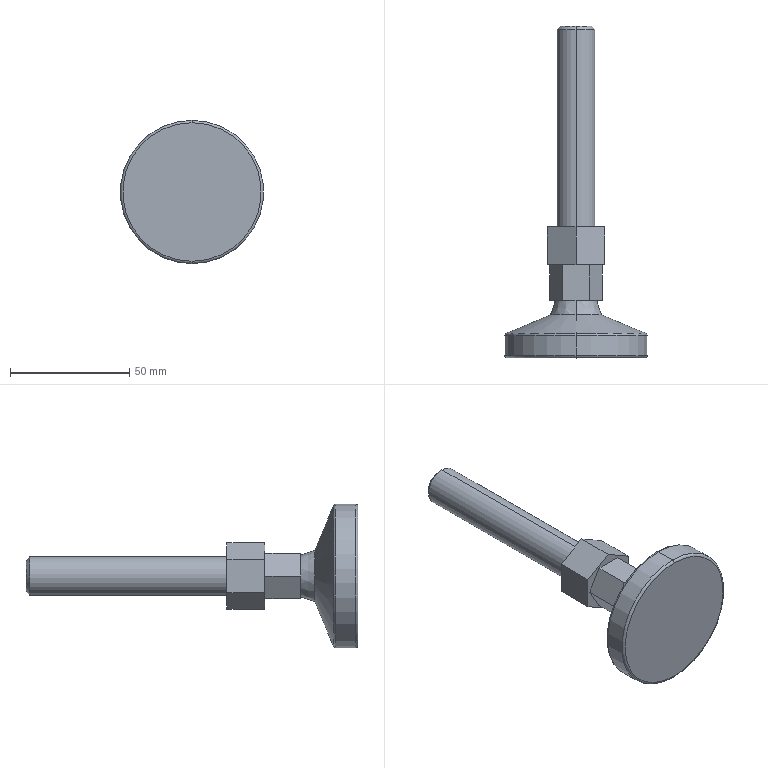Part | STEP file | All-carbon-steel swivel leveling foot KCUF M16-100-60-electrophoretic black | 1 solid | 31 faces | box 60 x 139 x 60 mm | volume 70730 mm3 | plane 17 | cone 6 | torus 4 | cylinder 4 | commonest cylinder face diameters 16 x2 60 x2